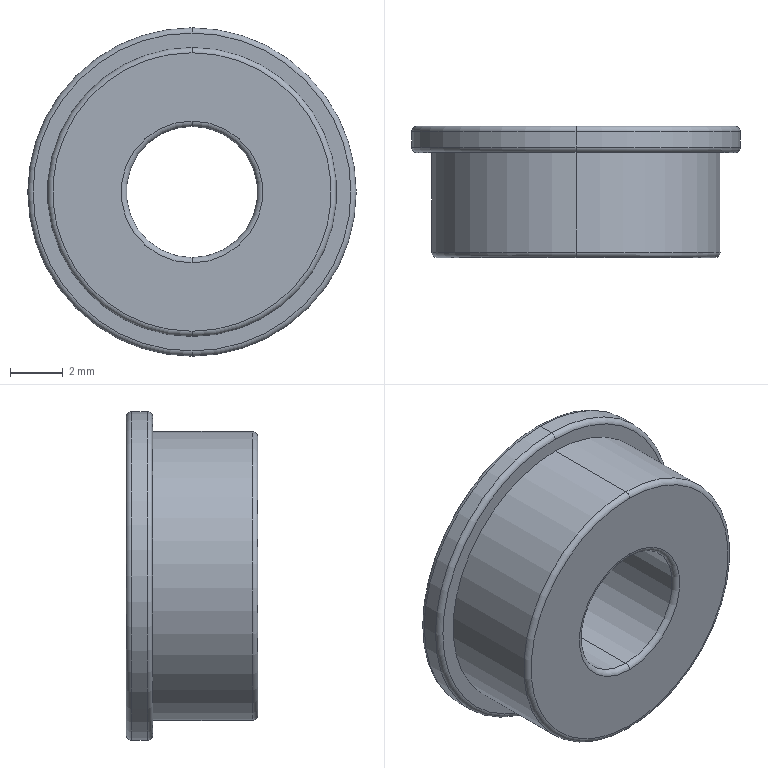Part | NX | features BREP 1 | 1 solid | 19 faces | box 12.5 x 5 x 12.5 mm | volume 403.438 mm3 | torus 10 | cylinder 6 | plane 3 | commonest cylinder face diameters 5 x2 11 x2 12.5 x2
STEP:
#1=CARTESIAN_POINT('',(0.,4.8,2.5));
#2=VERTEX_POINT('',#1);
#3=CARTESIAN_POINT('',(0.,5.,2.7));
#4=VERTEX_POINT('',#3);
#5=CARTESIAN_POINT('',(0.,4.8,2.7));
#6=DIRECTION('',(1.,0.,0.));
#7=DIRECTION('',(0.,0.,-1.));
#8=AXIS2_PLACEMENT_3D('',#5,#6,#7);
#9=CIRCLE('',#8,0.2);
#10=EDGE_CURVE('',#2,#4,#9,.T.);
#11=ORIENTED_EDGE('',*,*,#10,.F.);
#12=CARTESIAN_POINT('',(0.,4.8,-2.5));
#13=VERTEX_POINT('',#12);
#14=CARTESIAN_POINT('',(0.,4.8,0.));
#15=DIRECTION('',(0.,1.,0.));
#16=DIRECTION('',(0.,0.,-1.));
#17=AXIS2_PLACEMENT_3D('',#14,#15,#16);
#18=CIRCLE('',#17,2.5);
#19=EDGE_CURVE('',#13,#2,#18,.T.);
#20=ORIENTED_EDGE('',*,*,#19,.F.);
#21=CARTESIAN_POINT('',(0.,5.,-2.7));
#22=VERTEX_POINT('',#21);
#23=CARTESIAN_POINT('',(0.,4.8,-2.7));
#24=DIRECTION('',(-1.,0.,0.));
#25=DIRECTION('',(0.,0.,1.));
#26=AXIS2_PLACEMENT_3D('',#23,#24,#25);
#27=CIRCLE('',#26,0.2);
#28=EDGE_CURVE('',#13,#22,#27,.T.);
#29=ORIENTED_EDGE('',*,*,#28,.T.);
#30=CARTESIAN_POINT('',(0.,5.,0.));
#31=DIRECTION('',(0.,-1.,0.));
#32=DIRECTION('',(0.,0.,-1.));
#33=AXIS2_PLACEMENT_3D('',#30,#31,#32);
#34=CIRCLE('',#33,2.7);
#35=EDGE_CURVE('',#4,#22,#34,.T.);
#36=ORIENTED_EDGE('',*,*,#35,.F.);
#37=EDGE_LOOP('',(#11,#20,#29,#36));
#38=FACE_BOUND('',#37,.T.);
#39=CARTESIAN_POINT('',(0.,4.8,0.));
#40=DIRECTION('',(0.,-1.,0.));
#41=DIRECTION('',(0.,0.,-1.));
#42=AXIS2_PLACEMENT_3D('',#39,#40,#41);
#43=TOROIDAL_SURFACE('',#42,2.7,0.2);
#44=ADVANCED_FACE('',(#38),#43,.T.);
#45=CARTESIAN_POINT('',(0.,5.,6.05));
#46=VERTEX_POINT('',#45);
#47=CARTESIAN_POINT('',(0.,4.8,6.25));
#48=VERTEX_POINT('',#47);
#49=CARTESIAN_POINT('',(0.,4.8,6.05));
#50=DIRECTION('',(1.,0.,0.));
#51=DIRECTION('',(0.,0.,-1.));
#52=AXIS2_PLACEMENT_3D('',#49,#50,#51);
#53=CIRCLE('',#52,0.2);
#54=EDGE_CURVE('',#46,#48,#53,.T.);
#55=ORIENTED_EDGE('',*,*,#54,.F.);
#56=CARTESIAN_POINT('',(0.,5.,-6.05));
#57=VERTEX_POINT('',#56);
#58=CARTESIAN_POINT('',(0.,5.,0.));
#59=DIRECTION('',(0.,1.,0.));
#60=DIRECTION('',(0.,0.,-1.));
#61=AXIS2_PLACEMENT_3D('',#58,#59,#60);
#62=CIRCLE('',#61,6.05);
#63=EDGE_CURVE('',#57,#46,#62,.T.);
#64=ORIENTED_EDGE('',*,*,#63,.F.);
#65=CARTESIAN_POINT('',(0.,4.8,-6.25));
#66=VERTEX_POINT('',#65);
#67=CARTESIAN_POINT('',(0.,4.8,-6.05));
#68=DIRECTION('',(-1.,0.,0.));
#69=DIRECTION('',(0.,0.,1.));
#70=AXIS2_PLACEMENT_3D('',#67,#68,#69);
#71=CIRCLE('',#70,0.2);
#72=EDGE_CURVE('',#57,#66,#71,.T.);
#73=ORIENTED_EDGE('',*,*,#72,.T.);
#74=CARTESIAN_POINT('',(0.,4.8,0.));
#75=DIRECTION('',(0.,-1.,0.));
#76=DIRECTION('',(0.,0.,-1.));
#77=AXIS2_PLACEMENT_3D('',#74,#75,#76);
#78=CIRCLE('',#77,6.25);
#79=EDGE_CURVE('',#48,#66,#78,.T.);
#80=ORIENTED_EDGE('',*,*,#79,.F.);
#81=EDGE_LOOP('',(#55,#64,#73,#80));
#82=FACE_BOUND('',#81,.T.);
#83=CARTESIAN_POINT('',(0.,4.8,0.));
#84=DIRECTION('',(0.,-1.,0.));
#85=DIRECTION('',(0.,0.,-1.));
#86=AXIS2_PLACEMENT_3D('',#83,#84,#85);
#87=TOROIDAL_SURFACE('',#86,6.05,0.2);
#88=ADVANCED_FACE('',(#82),#87,.T.);
#89=CARTESIAN_POINT('',(0.,4.2,-6.25));
#90=VERTEX_POINT('',#89);
#91=CARTESIAN_POINT('',(0.,4.,-6.05));
#92=VERTEX_POINT('',#91);
#93=CARTESIAN_POINT('',(0.,4.2,-6.05));
#94=DIRECTION('',(1.,0.,0.));
#95=DIRECTION('',(0.,0.,-1.));
#96=AXIS2_PLACEMENT_3D('',#93,#94,#95);
#97=CIRCLE('',#96,0.2);
#98=EDGE_CURVE('',#90,#92,#97,.F.);
#99=ORIENTED_EDGE('',*,*,#98,.T.);
#100=CARTESIAN_POINT('',(0.,4.,6.05));
#101=VERTEX_POINT('',#100);
#102=CARTESIAN_POINT('',(0.,4.,0.));
#103=DIRECTION('',(0.,-1.,0.));
#104=DIRECTION('',(0.,0.,1.));
#105=AXIS2_PLACEMENT_3D('',#102,#103,#104);
#106=CIRCLE('',#105,6.05);
#107=EDGE_CURVE('',#101,#92,#106,.T.);
#108=ORIENTED_EDGE('',*,*,#107,.F.);
#109=CARTESIAN_POINT('',(0.,4.2,6.25));
#110=VERTEX_POINT('',#109);
#111=CARTESIAN_POINT('',(0.,4.2,6.05));
#112=DIRECTION('',(-1.,0.,0.));
#113=DIRECTION('',(0.,0.,1.));
#114=AXIS2_PLACEMENT_3D('',#111,#112,#113);
#115=CIRCLE('',#114,0.2);
#116=EDGE_CURVE('',#110,#101,#115,.F.);
#117=ORIENTED_EDGE('',*,*,#116,.F.);
#118=CARTESIAN_POINT('',(0.,4.2,0.));
#119=DIRECTION('',(0.,1.,0.));
#120=DIRECTION('',(0.,0.,1.));
#121=AXIS2_PLACEMENT_3D('',#118,#119,#120);
#122=CIRCLE('',#121,6.25);
#123=EDGE_CURVE('',#90,#110,#122,.T.);
#124=ORIENTED_EDGE('',*,*,#123,.F.);
#125=EDGE_LOOP('',(#99,#108,#117,#124));
#126=FACE_BOUND('',#125,.T.);
#127=CARTESIAN_POINT('',(0.,4.2,0.));
#128=DIRECTION('',(0.,1.,0.));
#129=DIRECTION('',(0.,0.,1.));
#130=AXIS2_PLACEMENT_3D('',#127,#128,#129);
#131=TOROIDAL_SURFACE('',#130,6.05,0.2);
#132=ADVANCED_FACE('',(#126),#131,.T.);
#133=CARTESIAN_POINT('',(0.,0.2,-5.5));
#134=VERTEX_POINT('',#133);
#135=CARTESIAN_POINT('',(0.,0.,-5.3));
#136=VERTEX_POINT('',#135);
#137=CARTESIAN_POINT('',(0.,0.2,-5.3));
#138=DIRECTION('',(1.,0.,0.));
#139=DIRECTION('',(0.,0.,-1.));
#140=AXIS2_PLACEMENT_3D('',#137,#138,#139);
#141=CIRCLE('',#140,0.2);
#142=EDGE_CURVE('',#134,#136,#141,.F.);
#143=ORIENTED_EDGE('',*,*,#142,.T.);
#144=CARTESIAN_POINT('',(0.,0.,5.3));
#145=VERTEX_POINT('',#144);
#146=CARTESIAN_POINT('',(0.,0.,0.));
#147=DIRECTION('',(0.,-1.,0.));
#148=DIRECTION('',(0.,0.,1.));
#149=AXIS2_PLACEMENT_3D('',#146,#147,#148);
#150=CIRCLE('',#149,5.3);
#151=EDGE_CURVE('',#145,#136,#150,.T.);
#152=ORIENTED_EDGE('',*,*,#151,.F.);
#153=CARTESIAN_POINT('',(0.,0.2,5.5));
#154=VERTEX_POINT('',#153);
#155=CARTESIAN_POINT('',(0.,0.2,5.3));
#156=DIRECTION('',(-1.,0.,0.));
#157=DIRECTION('',(0.,0.,1.));
#158=AXIS2_PLACEMENT_3D('',#155,#156,#157);
#159=CIRCLE('',#158,0.2);
#160=EDGE_CURVE('',#154,#145,#159,.F.);
#161=ORIENTED_EDGE('',*,*,#160,.F.);
#162=CARTESIAN_POINT('',(0.,0.2,0.));
#163=DIRECTION('',(0.,1.,0.));
#164=DIRECTION('',(0.,0.,1.));
#165=AXIS2_PLACEMENT_3D('',#162,#163,#164);
#166=CIRCLE('',#165,5.5);
#167=EDGE_CURVE('',#134,#154,#166,.T.);
#168=ORIENTED_EDGE('',*,*,#167,.F.);
#169=EDGE_LOOP('',(#143,#152,#161,#168));
#170=FACE_BOUND('',#169,.T.);
#171=CARTESIAN_POINT('',(0.,0.2,0.));
#172=DIRECTION('',(0.,1.,0.));
#173=DIRECTION('',(0.,0.,1.));
#174=AXIS2_PLACEMENT_3D('',#171,#172,#173);
#175=TOROIDAL_SURFACE('',#174,5.3,0.2);
#176=ADVANCED_FACE('',(#170),#175,.T.);
#177=CARTESIAN_POINT('',(0.,0.,-2.7));
#178=VERTEX_POINT('',#177);
#179=CARTESIAN_POINT('',(0.,0.2,-2.5));
#180=VERTEX_POINT('',#179);
#181=CARTESIAN_POINT('',(0.,0.2,-2.7));
#182=DIRECTION('',(1.,0.,0.));
#183=DIRECTION('',(0.,0.,-1.));
#184=AXIS2_PLACEMENT_3D('',#181,#182,#183);
#185=CIRCLE('',#184,0.2);
#186=EDGE_CURVE('',#178,#180,#185,.F.);
#187=ORIENTED_EDGE('',*,*,#186,.T.);
#188=CARTESIAN_POINT('',(0.,0.2,2.5));
#189=VERTEX_POINT('',#188);
#190=CARTESIAN_POINT('',(0.,0.2,0.));
#191=DIRECTION('',(0.,-1.,0.));
#192=DIRECTION('',(0.,0.,1.));
#193=AXIS2_PLACEMENT_3D('',#190,#191,#192);
#194=CIRCLE('',#193,2.5);
#195=EDGE_CURVE('',#189,#180,#194,.T.);
#196=ORIENTED_EDGE('',*,*,#195,.F.);
#197=CARTESIAN_POINT('',(0.,0.,2.7));
#198=VERTEX_POINT('',#197);
#199=CARTESIAN_POINT('',(0.,0.2,2.7));
#200=DIRECTION('',(-1.,0.,0.));
#201=DIRECTION('',(0.,0.,1.));
#202=AXIS2_PLACEMENT_3D('',#199,#200,#201);
#203=CIRCLE('',#202,0.2);
#204=EDGE_CURVE('',#198,#189,#203,.F.);
#205=ORIENTED_EDGE('',*,*,#204,.F.);
#206=CARTESIAN_POINT('',(0.,0.,0.));
#207=DIRECTION('',(0.,1.,0.));
#208=DIRECTION('',(0.,0.,1.));
#209=AXIS2_PLACEMENT_3D('',#206,#207,#208);
#210=CIRCLE('',#209,2.7);
#211=EDGE_CURVE('',#178,#198,#210,.T.);
#212=ORIENTED_EDGE('',*,*,#211,.F.);
#213=EDGE_LOOP('',(#187,#196,#205,#212));
#214=FACE_BOUND('',#213,.T.);
#215=CARTESIAN_POINT('',(0.,0.2,0.));
#216=DIRECTION('',(0.,1.,0.));
#217=DIRECTION('',(0.,0.,1.));
#218=AXIS2_PLACEMENT_3D('',#215,#216,#217);
#219=TOROIDAL_SURFACE('',#218,2.7,0.2);
#220=ADVANCED_FACE('',(#214),#219,.T.);
#221=ORIENTED_EDGE('',*,*,#151,.T.);
#222=CARTESIAN_POINT('',(0.,0.,0.));
#223=DIRECTION('',(0.,-1.,0.));
#224=DIRECTION('',(0.,0.,1.));
#225=AXIS2_PLACEMENT_3D('',#222,#223,#224);
#226=CIRCLE('',#225,5.3);
#227=EDGE_CURVE('',#136,#145,#226,.T.);
#228=ORIENTED_EDGE('',*,*,#227,.T.);
#229=EDGE_LOOP('',(#221,#228));
#230=FACE_BOUND('',#229,.T.);
#231=CARTESIAN_POINT('',(0.,0.,0.));
#232=DIRECTION('',(0.,1.,0.));
#233=DIRECTION('',(0.,0.,1.));
#234=AXIS2_PLACEMENT_3D('',#231,#232,#233);
#235=CIRCLE('',#234,2.7);
#236=EDGE_CURVE('',#198,#178,#235,.T.);
#237=ORIENTED_EDGE('',*,*,#236,.T.);
#238=ORIENTED_EDGE('',*,*,#211,.T.);
#239=EDGE_LOOP('',(#237,#238));
#240=FACE_BOUND('',#239,.T.);
#241=CARTESIAN_POINT('',(-5.5,0.,0.));
#242=DIRECTION('',(0.,1.,0.));
#243=DIRECTION('',(0.,0.,1.));
#244=AXIS2_PLACEMENT_3D('',#241,#242,#243);
#245=PLANE('',#244);
#246=ADVANCED_FACE('',(#230,#240),#245,.F.);
#247=CARTESIAN_POINT('',(0.,4.,5.5));
#248=VERTEX_POINT('',#247);
#249=CARTESIAN_POINT('',(0.,0.,5.5));
#250=DIRECTION('',(0.,-1.,0.));
#251=VECTOR('',#250,1000.);
#252=LINE('',#249,#251);
#253=EDGE_CURVE('',#248,#154,#252,.T.);
#254=ORIENTED_EDGE('',*,*,#253,.F.);
#255=CARTESIAN_POINT('',(0.,4.,-5.5));
#256=VERTEX_POINT('',#255);
#257=CARTESIAN_POINT('',(0.,4.,0.));
#258=DIRECTION('',(0.,-1.,0.));
#259=DIRECTION('',(0.,0.,-1.));
#260=AXIS2_PLACEMENT_3D('',#257,#258,#259);
#261=CIRCLE('',#260,5.5);
#262=EDGE_CURVE('',#248,#256,#261,.T.);
#263=ORIENTED_EDGE('',*,*,#262,.T.);
#264=CARTESIAN_POINT('',(0.,0.,-5.5));
#265=DIRECTION('',(0.,-1.,0.));
#266=VECTOR('',#265,1000.);
#267=LINE('',#264,#266);
#268=EDGE_CURVE('',#256,#134,#267,.T.);
#269=ORIENTED_EDGE('',*,*,#268,.T.);
#270=ORIENTED_EDGE('',*,*,#167,.T.);
#271=EDGE_LOOP('',(#254,#263,#269,#270));
#272=FACE_BOUND('',#271,.T.);
#273=CARTESIAN_POINT('',(0.,0.,0.));
#274=DIRECTION('',(0.,-1.,0.));
#275=DIRECTION('',(0.,0.,-1.));
#276=AXIS2_PLACEMENT_3D('',#273,#274,#275);
#277=CYLINDRICAL_SURFACE('',#276,5.5);
#278=ADVANCED_FACE('',(#272),#277,.T.);
#279=CARTESIAN_POINT('',(0.,4.,0.));
#280=DIRECTION('',(0.,-1.,0.));
#281=DIRECTION('',(0.,0.,-1.));
#282=AXIS2_PLACEMENT_3D('',#279,#280,#281);
#283=CIRCLE('',#282,5.5);
#284=EDGE_CURVE('',#256,#248,#283,.T.);
#285=ORIENTED_EDGE('',*,*,#284,.F.);
#286=ORIENTED_EDGE('',*,*,#262,.F.);
#287=EDGE_LOOP('',(#285,#286));
#288=FACE_BOUND('',#287,.T.);
#289=ORIENTED_EDGE('',*,*,#107,.T.);
#290=CARTESIAN_POINT('',(0.,4.,0.));
#291=DIRECTION('',(0.,-1.,0.));
#292=DIRECTION('',(0.,0.,1.));
#293=AXIS2_PLACEMENT_3D('',#290,#291,#292);
#294=CIRCLE('',#293,6.05);
#295=EDGE_CURVE('',#92,#101,#294,.T.);
#296=ORIENTED_EDGE('',*,*,#295,.T.);
#297=EDGE_LOOP('',(#289,#296));
#298=FACE_BOUND('',#297,.T.);
#299=CARTESIAN_POINT('',(-6.25,4.,0.));
#300=DIRECTION('',(0.,1.,0.));
#301=DIRECTION('',(0.,0.,1.));
#302=AXIS2_PLACEMENT_3D('',#299,#300,#301);
#303=PLANE('',#302);
#304=ADVANCED_FACE('',(#288,#298),#303,.F.);
#305=CARTESIAN_POINT('',(0.,0.,6.25));
#306=DIRECTION('',(0.,-1.,0.));
#307=VECTOR('',#306,1000.);
#308=LINE('',#305,#307);
#309=EDGE_CURVE('',#48,#110,#308,.T.);
#310=ORIENTED_EDGE('',*,*,#309,.F.);
#311=ORIENTED_EDGE('',*,*,#79,.T.);
#312=CARTESIAN_POINT('',(0.,0.,-6.25));
#313=DIRECTION('',(0.,-1.,0.));
#314=VECTOR('',#313,1000.);
#315=LINE('',#312,#314);
#316=EDGE_CURVE('',#66,#90,#315,.T.);
#317=ORIENTED_EDGE('',*,*,#316,.T.);
#318=ORIENTED_EDGE('',*,*,#123,.T.);
#319=EDGE_LOOP('',(#310,#311,#317,#318));
#320=FACE_BOUND('',#319,.T.);
#321=CARTESIAN_POINT('',(0.,0.,0.));
#322=DIRECTION('',(0.,-1.,0.));
#323=DIRECTION('',(0.,0.,-1.));
#324=AXIS2_PLACEMENT_3D('',#321,#322,#323);
#325=CYLINDRICAL_SURFACE('',#324,6.25);
#326=ADVANCED_FACE('',(#320),#325,.T.);
#327=CARTESIAN_POINT('',(0.,5.,0.));
#328=DIRECTION('',(0.,-1.,0.));
#329=DIRECTION('',(0.,0.,-1.));
#330=AXIS2_PLACEMENT_3D('',#327,#328,#329);
#331=CIRCLE('',#330,2.7);
#332=EDGE_CURVE('',#22,#4,#331,.T.);
#333=ORIENTED_EDGE('',*,*,#332,.T.);
#334=ORIENTED_EDGE('',*,*,#35,.T.);
#335=EDGE_LOOP('',(#333,#334));
#336=FACE_BOUND('',#335,.T.);
#337=ORIENTED_EDGE('',*,*,#63,.T.);
#338=CARTESIAN_POINT('',(0.,5.,0.));
#339=DIRECTION('',(0.,1.,0.));
#340=DIRECTION('',(0.,0.,-1.));
#341=AXIS2_PLACEMENT_3D('',#338,#339,#340);
#342=CIRCLE('',#341,6.05);
#343=EDGE_CURVE('',#46,#57,#342,.T.);
#344=ORIENTED_EDGE('',*,*,#343,.T.);
#345=EDGE_LOOP('',(#337,#344));
#346=FACE_BOUND('',#345,.T.);
#347=CARTESIAN_POINT('',(-2.5,5.,0.));
#348=DIRECTION('',(0.,-1.,0.));
#349=DIRECTION('',(0.,0.,-1.));
#350=AXIS2_PLACEMENT_3D('',#347,#348,#349);
#351=PLANE('',#350);
#352=ADVANCED_FACE('',(#336,#346),#351,.F.);
#353=CARTESIAN_POINT('',(0.,0.,2.5));
#354=DIRECTION('',(0.,-1.,0.));
#355=VECTOR('',#354,1000.);
#356=LINE('',#353,#355);
#357=EDGE_CURVE('',#2,#189,#356,.T.);
#358=ORIENTED_EDGE('',*,*,#357,.F.);
#359=CARTESIAN_POINT('',(0.,4.8,0.));
#360=DIRECTION('',(0.,1.,0.));
#361=DIRECTION('',(0.,0.,-1.));
#362=AXIS2_PLACEMENT_3D('',#359,#360,#361);
#363=CIRCLE('',#362,2.5);
#364=EDGE_CURVE('',#2,#13,#363,.T.);
#365=ORIENTED_EDGE('',*,*,#364,.T.);
#366=CARTESIAN_POINT('',(0.,0.,-2.5));
#367=DIRECTION('',(0.,-1.,0.));
#368=VECTOR('',#367,1000.);
#369=LINE('',#366,#368);
#370=EDGE_CURVE('',#13,#180,#369,.T.);
#371=ORIENTED_EDGE('',*,*,#370,.T.);
#372=CARTESIAN_POINT('',(0.,0.2,0.));
#373=DIRECTION('',(0.,-1.,0.));
#374=DIRECTION('',(0.,0.,1.));
#375=AXIS2_PLACEMENT_3D('',#372,#373,#374);
#376=CIRCLE('',#375,2.5);
#377=EDGE_CURVE('',#180,#189,#376,.T.);
#378=ORIENTED_EDGE('',*,*,#377,.T.);
#379=EDGE_LOOP('',(#358,#365,#371,#378));
#380=FACE_BOUND('',#379,.T.);
#381=CARTESIAN_POINT('',(0.,0.,0.));
#382=DIRECTION('',(0.,-1.,0.));
#383=DIRECTION('',(0.,0.,-1.));
#384=AXIS2_PLACEMENT_3D('',#381,#382,#383);
#385=CYLINDRICAL_SURFACE('',#384,2.5);
#386=ADVANCED_FACE('',(#380),#385,.F.);
#387=ORIENTED_EDGE('',*,*,#19,.T.);
#388=ORIENTED_EDGE('',*,*,#357,.T.);
#389=ORIENTED_EDGE('',*,*,#195,.T.);
#390=ORIENTED_EDGE('',*,*,#370,.F.);
#391=EDGE_LOOP('',(#387,#388,#389,#390));
#392=FACE_BOUND('',#391,.T.);
#393=CARTESIAN_POINT('',(0.,0.,0.));
#394=DIRECTION('',(0.,-1.,0.));
#395=DIRECTION('',(0.,0.,-1.));
#396=AXIS2_PLACEMENT_3D('',#393,#394,#395);
#397=CYLINDRICAL_SURFACE('',#396,2.5);
#398=ADVANCED_FACE('',(#392),#397,.F.);
#399=CARTESIAN_POINT('',(0.,4.8,0.));
#400=DIRECTION('',(0.,-1.,0.));
#401=DIRECTION('',(0.,0.,-1.));
#402=AXIS2_PLACEMENT_3D('',#399,#400,#401);
#403=CIRCLE('',#402,6.25);
#404=EDGE_CURVE('',#66,#48,#403,.T.);
#405=ORIENTED_EDGE('',*,*,#404,.T.);
#406=ORIENTED_EDGE('',*,*,#309,.T.);
#407=CARTESIAN_POINT('',(0.,4.2,0.));
#408=DIRECTION('',(0.,1.,0.));
#409=DIRECTION('',(0.,0.,1.));
#410=AXIS2_PLACEMENT_3D('',#407,#408,#409);
#411=CIRCLE('',#410,6.25);
#412=EDGE_CURVE('',#110,#90,#411,.T.);
#413=ORIENTED_EDGE('',*,*,#412,.T.);
#414=ORIENTED_EDGE('',*,*,#316,.F.);
#415=EDGE_LOOP('',(#405,#406,#413,#414));
#416=FACE_BOUND('',#415,.T.);
#417=CARTESIAN_POINT('',(0.,0.,0.));
#418=DIRECTION('',(0.,-1.,0.));
#419=DIRECTION('',(0.,0.,-1.));
#420=AXIS2_PLACEMENT_3D('',#417,#418,#419);
#421=CYLINDRICAL_SURFACE('',#420,6.25);
#422=ADVANCED_FACE('',(#416),#421,.T.);
#423=ORIENTED_EDGE('',*,*,#284,.T.);
#424=ORIENTED_EDGE('',*,*,#253,.T.);
#425=CARTESIAN_POINT('',(0.,0.2,0.));
#426=DIRECTION('',(0.,1.,0.));
#427=DIRECTION('',(0.,0.,1.));
#428=AXIS2_PLACEMENT_3D('',#425,#426,#427);
#429=CIRCLE('',#428,5.5);
#430=EDGE_CURVE('',#154,#134,#429,.T.);
#431=ORIENTED_EDGE('',*,*,#430,.T.);
#432=ORIENTED_EDGE('',*,*,#268,.F.);
#433=EDGE_LOOP('',(#423,#424,#431,#432));
#434=FACE_BOUND('',#433,.T.);
#435=CARTESIAN_POINT('',(0.,0.,0.));
#436=DIRECTION('',(0.,-1.,0.));
#437=DIRECTION('',(0.,0.,-1.));
#438=AXIS2_PLACEMENT_3D('',#435,#436,#437);
#439=CYLINDRICAL_SURFACE('',#438,5.5);
#440=ADVANCED_FACE('',(#434),#439,.T.);
#441=ORIENTED_EDGE('',*,*,#377,.F.);
#442=ORIENTED_EDGE('',*,*,#186,.F.);
#443=ORIENTED_EDGE('',*,*,#236,.F.);
#444=ORIENTED_EDGE('',*,*,#204,.T.);
#445=EDGE_LOOP('',(#441,#442,#443,#444));
#446=FACE_BOUND('',#445,.T.);
#447=CARTESIAN_POINT('',(0.,0.2,0.));
#448=DIRECTION('',(0.,1.,0.));
#449=DIRECTION('',(0.,0.,1.));
#450=AXIS2_PLACEMENT_3D('',#447,#448,#449);
#451=TOROIDAL_SURFACE('',#450,2.7,0.2);
#452=ADVANCED_FACE('',(#446),#451,.T.);
#453=ORIENTED_EDGE('',*,*,#227,.F.);
#454=ORIENTED_EDGE('',*,*,#142,.F.);
#455=ORIENTED_EDGE('',*,*,#430,.F.);
#456=ORIENTED_EDGE('',*,*,#160,.T.);
#457=EDGE_LOOP('',(#453,#454,#455,#456));
#458=FACE_BOUND('',#457,.T.);
#459=CARTESIAN_POINT('',(0.,0.2,0.));
#460=DIRECTION('',(0.,1.,0.));
#461=DIRECTION('',(0.,0.,1.));
#462=AXIS2_PLACEMENT_3D('',#459,#460,#461);
#463=TOROIDAL_SURFACE('',#462,5.3,0.2);
#464=ADVANCED_FACE('',(#458),#463,.T.);
#465=ORIENTED_EDGE('',*,*,#295,.F.);
#466=ORIENTED_EDGE('',*,*,#98,.F.);
#467=ORIENTED_EDGE('',*,*,#412,.F.);
#468=ORIENTED_EDGE('',*,*,#116,.T.);
#469=EDGE_LOOP('',(#465,#466,#467,#468));
#470=FACE_BOUND('',#469,.T.);
#471=CARTESIAN_POINT('',(0.,4.2,0.));
#472=DIRECTION('',(0.,1.,0.));
#473=DIRECTION('',(0.,0.,1.));
#474=AXIS2_PLACEMENT_3D('',#471,#472,#473);
#475=TOROIDAL_SURFACE('',#474,6.05,0.2);
#476=ADVANCED_FACE('',(#470),#475,.T.);
#477=ORIENTED_EDGE('',*,*,#343,.F.);
#478=ORIENTED_EDGE('',*,*,#54,.T.);
#479=ORIENTED_EDGE('',*,*,#404,.F.);
#480=ORIENTED_EDGE('',*,*,#72,.F.);
#481=EDGE_LOOP('',(#477,#478,#479,#480));
#482=FACE_BOUND('',#481,.T.);
#483=CARTESIAN_POINT('',(0.,4.8,0.));
#484=DIRECTION('',(0.,-1.,0.));
#485=DIRECTION('',(0.,0.,-1.));
#486=AXIS2_PLACEMENT_3D('',#483,#484,#485);
#487=TOROIDAL_SURFACE('',#486,6.05,0.2);
#488=ADVANCED_FACE('',(#482),#487,.T.);
#489=ORIENTED_EDGE('',*,*,#364,.F.);
#490=ORIENTED_EDGE('',*,*,#10,.T.);
#491=ORIENTED_EDGE('',*,*,#332,.F.);
#492=ORIENTED_EDGE('',*,*,#28,.F.);
#493=EDGE_LOOP('',(#489,#490,#491,#492));
#494=FACE_BOUND('',#493,.T.);
#495=CARTESIAN_POINT('',(0.,4.8,0.));
#496=DIRECTION('',(0.,-1.,0.));
#497=DIRECTION('',(0.,0.,-1.));
#498=AXIS2_PLACEMENT_3D('',#495,#496,#497);
#499=TOROIDAL_SURFACE('',#498,2.7,0.2);
#500=ADVANCED_FACE('',(#494),#499,.T.);
#501=CLOSED_SHELL('',(#44,#88,#132,#176,#220,#246,#278,#304,#326,#352,#386,#398,#422,#440,#452,#464,#476,#488,#500));
#502=MANIFOLD_SOLID_BREP('',#501);
#503=(LENGTH_UNIT()NAMED_UNIT(*)SI_UNIT(.MILLI.,.METRE.));
#504=UNCERTAINTY_MEASURE_WITH_UNIT(LENGTH_MEASURE(0.00001),#503,'','');
#505=(NAMED_UNIT(*)PLANE_ANGLE_UNIT()SI_UNIT($,.RADIAN.));
#506=(NAMED_UNIT(*)SI_UNIT($,.STERADIAN.)SOLID_ANGLE_UNIT());
#507=(GEOMETRIC_REPRESENTATION_CONTEXT(3)GLOBAL_UNCERTAINTY_ASSIGNED_CONTEXT((#504))GLOBAL_UNIT_ASSIGNED_CONTEXT((#503,#505,#506))REPRESENTATION_CONTEXT('',''));
#508=ADVANCED_BREP_SHAPE_REPRESENTATION('',(#502),#507);